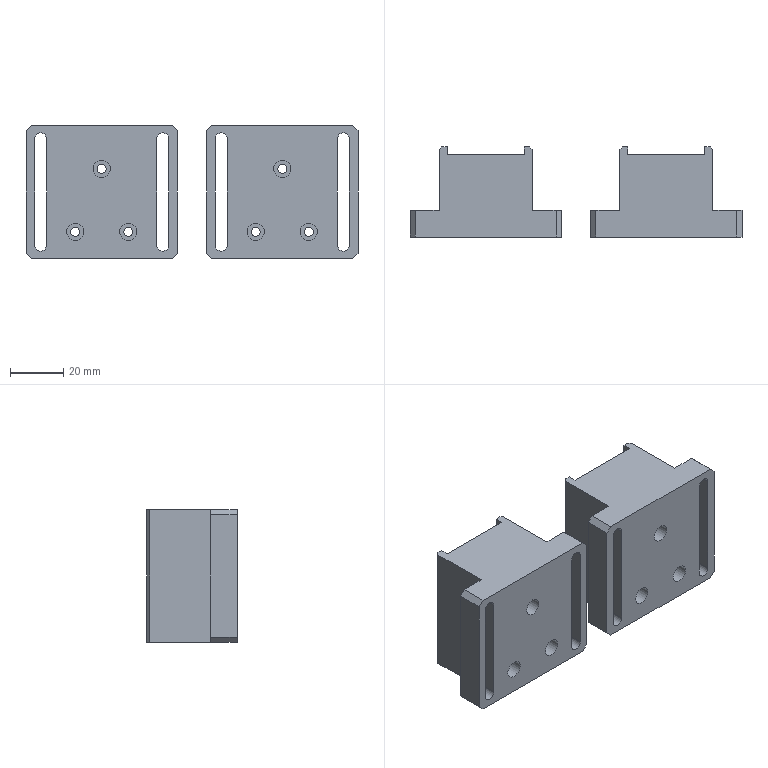CAM job | NX | 3+2 milling, drilling | part box 125 x 34 x 50 mm | stock box 129 x 40.5 x 55 mm
Tools:
number,name,description,diameter,corner_radius,flute_length,length,flutes
4,D4,平底铣刀-粗,4.0,0.0,25.0,75.0,2
9,D10,平底铣刀-粗,10.0,0.0,35.0,75.0,2
17,D4-J,平底铣刀-精,4.0,0.0,50.0,75.0,2
10,D10-J,平底铣刀-精,10.0,0.0,35.0,75.0,2
1,D80R0.8飞刀,圆鼻刀-粗,80.0,0.8,50.0,75.0,2
1,D80R0.8飞刀-J,圆鼻刀-精,80.0,0.8,50.0,75.0,2
2,D6倒角刀,倒角刀,6.0,0.0,3.0,25.0,2
13,ZT3.4,钻头,3.4,0.0,35.0,50.0,2
Operations:
program,operation,operation_type,tool,method,geometry_group,spindle_rpm,surface_speed,feed_per_tooth,feed_cut,feed_plunge,cut_length_mm,path_length_mm,cut_time_min,machine_time_min
B,底壁铣飞面开粗_COPY,VolumeBased25DMillingOperation,D80R0.8飞刀,分层开粗-切深K-步距G,W-B,5000.0,1256.637,0.25,2500.0,100.0,2798.328,5604.789,1.119,1.4
B,底壁铣飞面精光_COPY,VolumeBased25DMillingOperation,D80R0.8飞刀-J,侧刃精光-切深K-步距G,W-B,5000.0,1256.637,0.1,1000.0,100.0,232.998,268.998,0.233,0.2366
B,底壁铣分层开粗-中_COPY,VolumeBased25DMillingOperation,D10,分层开粗-切深K-步距G,W-B,8000.0,251.32,0.25,4000.0,100.0,2744.96,2858.146,0.6862,0.6976
B,底壁铣分层开粗-中_COPY_1,VolumeBased25DMillingOperation,D10,分层开粗-切深K-步距G,W-B,8000.0,251.32,0.25,4000.0,100.0,31412.53,31817.635,7.853,7.894
B,钻倒角_1,Operation,D6倒角刀,METHOD,W-B,8000.0,150.796,0.0625,1000.0,0.0,30.0,261.337,0.03,0.0531
B,平面去毛刺6X45L_COPY,SurfaceContour,D6倒角刀,爬面_倒角-切深0-步距G,W-B,6500.0,122.519,0.1154,1500.0,100.0,1227.156,2759.047,0.8181,0.9713
B,底壁铣倒角_COPY,VolumeBased25DMillingOperation,D6倒角刀,爬面_倒角-切深0-步距G,W-B,6500.0,122.519,0.1154,1500.0,100.0,235.202,501.218,0.1568,0.1834
B,底壁铣精光底面-中_COPY,VolumeBased25DMillingOperation,D10-J,精光步距切深关,W-B,7000.0,175.0,0.0536,1500.0,100.0,1430.534,1844.485,0.9537,0.9951
B,底壁铣精光侧面-中-选底面_COPY_1,VolumeBased25DMillingOperation,D10-J,侧刃精光-切深K-步距G,W-B,8000.0,251.32,0.0625,1000.0,100.0,549.455,983.421,0.5495,0.5929
B,底壁铣精光侧面-中-选底面_COPY,VolumeBased25DMillingOperation,D10-J,侧刃精光-切深K-步距G,W-B,8000.0,251.32,0.0625,1000.0,100.0,272.2,401.086,0.2722,0.2851
A,顶面,FaceMilling,D80R0.8飞刀,侧刃精光-切深K-步距G,W-A,4000.0,1005.31,0.125,1000.0,100.0,219.0,255.0,0.219,0.2226
A,外形粗_2,VolumeBased25DMillingOperation,D10,METHOD,W-A,8000.0,251.327,0.3125,5000.0,80.0,34275.902,34490.402,6.855,6.877
A,沉头孔打点-深0.8,Operation,D6倒角刀,NONE,W-A,8000.0,150.796,0.0312,500.0,90.0,25.2,627.42,0.0504,0.1106
A,沉头孔-钻孔0段,Operation,ZT3.4,NONE,W-A,2800.0,29.908,0.0536,300.0,90.0,322.3,1260.217,1.074,1.168
A,通腰槽粗_1,VolumeBased25DMillingOperation,D4,METHOD,W-A,8000.0,100.531,0.1562,2500.0,100.0,14899.482,15209.494,5.96,5.991
A,铣孔开粗D4_1,CylinderMilling,D4,NONE,W-A,8000.0,100.531,0.075,1200.0,100.0,3753.294,4279.741,3.128,3.18
A,铣孔精光D4_1,CylinderMilling,D4-J,精光步距切深关,W-A,8000.0,100.531,0.0312,500.0,100.0,355.064,881.511,0.7101,0.7628
A,腰槽精_1,VolumeBased25DMillingOperation,D4-J,METHOD,W-A,6000.0,113.0,0.0833,1000.0,100.0,1005.589,1430.807,1.006,1.048
A,仅选体,SurfaceContour,D6倒角刀,METHOD,W-A,8000.0,150.796,0.1875,3000.0,100.0,833.671,1263.288,0.2779,0.3209
A,铣倒角_1,PlanarMilling,D6倒角刀,NONE,W-A,8000.0,150.796,0.0312,500.0,100.0,175.533,530.236,0.3511,0.3865
A,外形半精_2,VolumeBased25DMillingOperation,D10-J,METHOD,W-A,8000.0,251.327,0.0625,1000.0,100.0,1495.136,2020.561,1.495,1.548